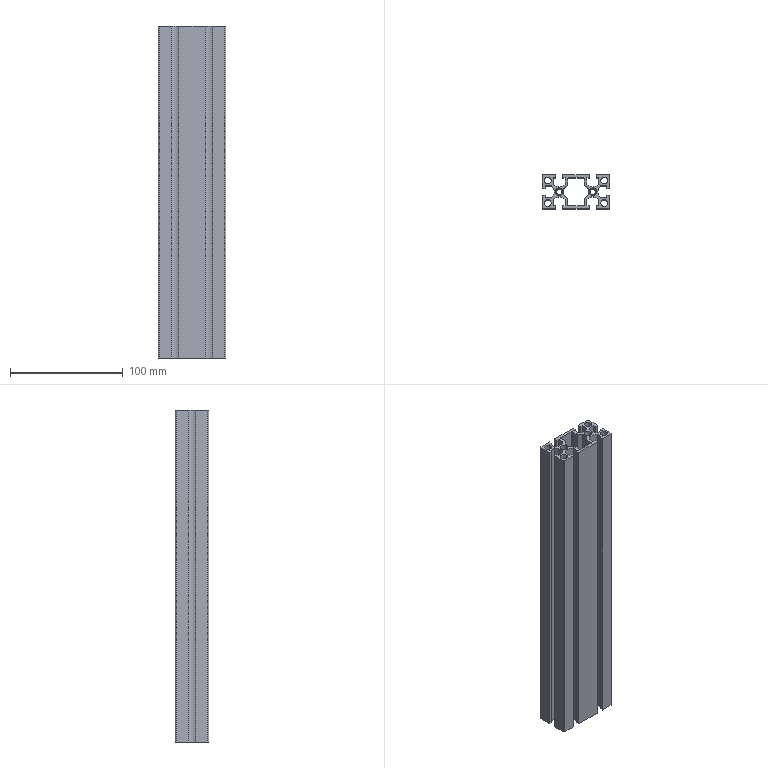Part | STEP file | 04-20 equal-height profile | 1 solid | 103 faces | box 60 x 30 x 295 mm | volume 194282 mm3 | plane 60 | cylinder 35 | cone 8 | commonest cylinder face diameters 2 x8 6 x8 6.8 x8 15 x7 5 x4